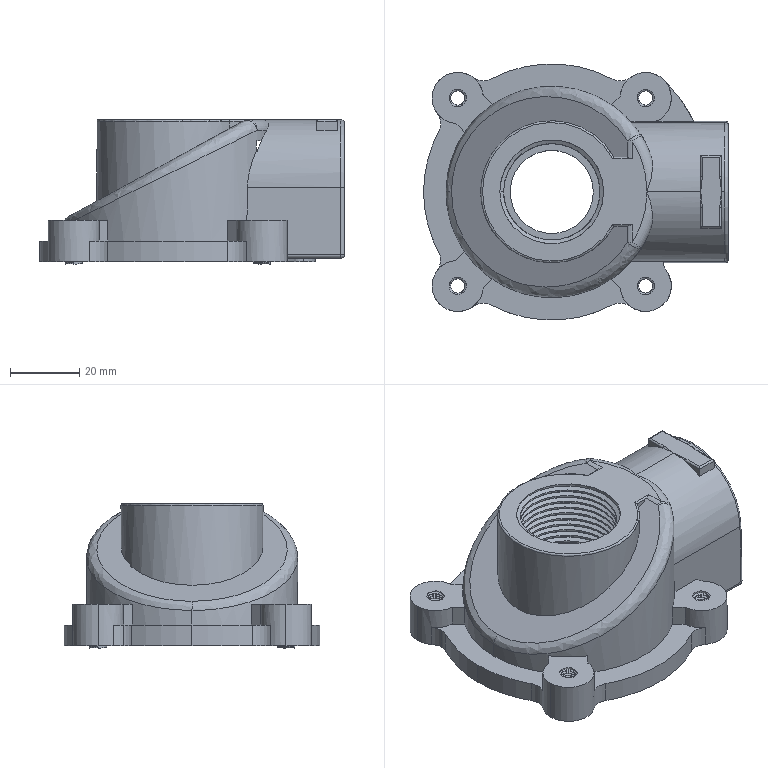Part | SolidWorks | features ICE 16, Fillet 11, CirPattern 3, SweepThread 3, Chamfer 1, Extrusion 1, Helix 1 | 1 solid | 329 faces | box 88 x 74 x 41.7 mm | volume 68269 mm3 | cylinder 234 | plane 51 | spline 31 | torus 5 | cone 4 | sphere 4 | commonest cylinder face diameters 5 x125 30 x50 10 x9 1 x8 4 x7 14.784 x6